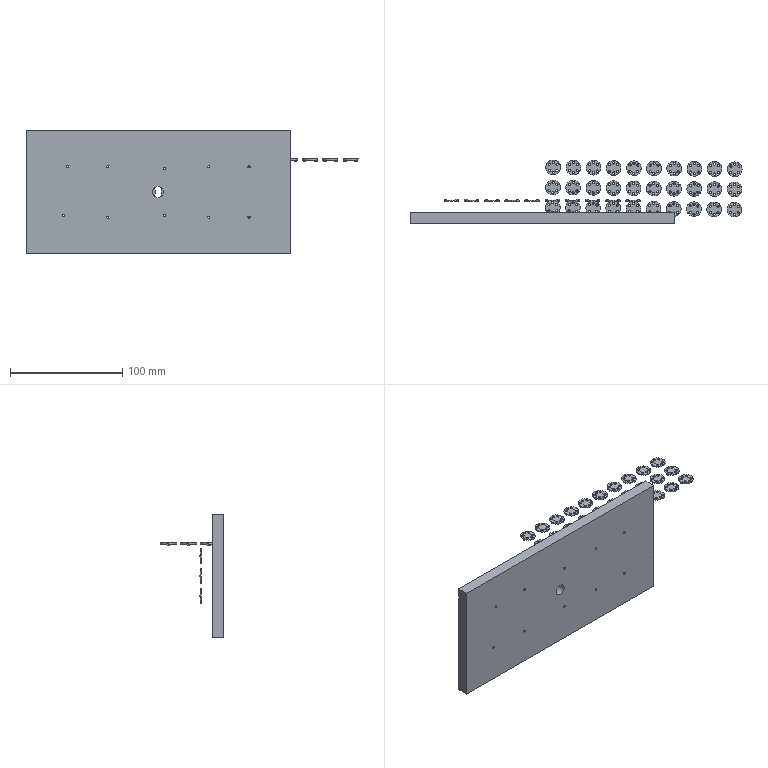CAM job | NX | 3+2 milling, drilling | part box 296.27 x 56.878 x 110 mm
Tools:
number,name,description,diameter,corner_radius,flute_length,length,flutes
0,D10R0,Milling Tool-5 Parameters,10.0,0.0,50.0,75.0,2
0,D3.R0,Milling Tool-5 Parameters,3.0,0.0,50.0,75.0,2
0,DK-Ø3,Countersink,3.0,0.0,0.0,60.0,2
0,D02钻头,Drilling Tool,2.0,0.0,35.0,50.0,2
0,D5R0,Milling Tool-5 Parameters,5.0,0.0,50.0,75.0,2
0,DJ-Ø3,Countersink,3.0,0.0,0.0,60.0,2
0,D2R0,Milling Tool-5 Parameters,2.0,0.0,50.0,75.0,2
0,DK-Ø6,Countersink,6.0,0.0,0.0,60.0,2
15,D16,Milling Tool-5 Parameters,16.0,0.0,50.0,75.0,2
9,D1,Milling Tool-5 Parameters,1.0,0.0,50.0,75.0,2
10,Z2.,Drilling Tool,2.0,0.0,35.0,50.0,2
Operations:
program,operation,operation_type,tool,method,geometry_group,spindle_rpm,surface_speed,feed_per_tooth,feed_cut,feed_plunge,cut_length_mm,path_length_mm,cut_time_min,machine_time_min
B01,FACE_MILLING_1,FaceMilling,D10R0,METHOD,WORKPIECE,2200.0,69.0,0.2727,1200.0,100.0,4849.667,5012.378,4.041,4.061
B02,FACE_MILLING_1_COPY,FaceMilling,D10R0,METHOD,WORKPIECE,2200.0,69.0,0.1818,800.0,100.0,1616.556,1637.456,2.021,2.024
B03,CAVITY_MILL_2,CavityMilling,D3.R0,METHOD,WORKPIECE,4000.0,50.0,0.25,2000.0,100.0,20644.369,20676.269,10.322,10.326
B04,DRILLING,Operation,DK-Ø3,METHOD,WORKPIECE,1500.0,14.0,0.0333,100.0,0.0,360.0,3355.57,3.6,3.9
B04,PLANAR_MILL_COPY_1_COPY_10,PlanarMilling,DK-Ø3,METHOD,WORKPIECE,5000.0,47.0,0.08,800.0,100.0,1403.867,2145.008,1.755,1.84
B05,DRILLING_COPY,Operation,D02钻头,METHOD,WORKPIECE,1500.0,14.0,0.0333,100.0,0.0,900.0,4435.57,9.0,9.354
B06,PLANAR_MILL_3,PlanarMilling,D16,METHOD,WORKPIECE,3500.0,175.0,0.0571,400.0,100.0,639.0,1096.562,1.597,1.643
A01,FACE_MILLING_1_COPY_1,FaceMilling,D10R0,METHOD,WORKPIECE_1,2200.0,69.0,0.2727,1200.0,100.0,4077.75,4637.993,3.398,3.461
A01,FACE_MILLING_1_COPY_1_COPY,FaceMilling,D10R0,METHOD,WORKPIECE_1,2500.0,78.0,0.14,700.0,100.0,1359.25,1459.25,1.942,1.957
A01,PLANAR_MILL_1,PlanarMilling,D10R0,METHOD,WORKPIECE_1,2500.0,78.0,0.14,700.0,100.0,2997.729,3611.928,4.282,4.344
A02,CAVITY_MILL_1_1,CavityMilling,D5R0,METHOD,WORKPIECE_1,4000.0,62.0,0.125,1000.0,100.0,21064.46,21624.203,21.064,21.123
A03,PLANAR_MILL_1_COPY_31,PlanarMilling,D1,METHOD,WORKPIECE_1,4500.0,14.0,0.0667,600.0,100.0,240.132,248.632,0.4002,0.4011
A03,PLANAR_MILL_1_COPY_COPY_30,PlanarMilling,D1,METHOD,WORKPIECE_1,4500.0,14.0,0.0667,600.0,100.0,240.132,248.632,0.4002,0.4011
A03,PLANAR_MILL_1_COPY_31_COPY_1,PlanarMilling,D1,METHOD,WORKPIECE_1,4500.0,14.0,0.0667,600.0,100.0,240.132,248.632,0.4002,0.4011
A03,PLANAR_MILL_1_COPY_COPY_30_COPY_1,PlanarMilling,D1,METHOD,WORKPIECE_1,4500.0,14.0,0.0667,600.0,100.0,240.132,248.632,0.4002,0.4011
A03,PLANAR_MILL_1_COPY_31_COPY_2,PlanarMilling,D1,METHOD,WORKPIECE_1,4500.0,14.0,0.0667,600.0,100.0,240.132,248.632,0.4002,0.4011
A03,PLANAR_MILL_1_COPY_COPY_30_COPY_2,PlanarMilling,D1,METHOD,WORKPIECE_1,4500.0,14.0,0.0667,600.0,100.0,240.132,248.632,0.4002,0.4011
A03,PLANAR_MILL_1_COPY_31_COPY_3,PlanarMilling,D1,METHOD,WORKPIECE_1,4500.0,14.0,0.0667,600.0,100.0,240.132,248.632,0.4002,0.4011
A03,PLANAR_MILL_1_COPY_COPY_30_COPY_3,PlanarMilling,D1,METHOD,WORKPIECE_1,4500.0,14.0,0.0667,600.0,100.0,240.132,248.632,0.4002,0.4011
A03,PLANAR_MILL_1_COPY_31_COPY_4,PlanarMilling,D1,METHOD,WORKPIECE_1,4500.0,14.0,0.0667,600.0,100.0,240.132,248.632,0.4002,0.4011
A03,PLANAR_MILL_1_COPY_COPY_30_COPY_4,PlanarMilling,D1,METHOD,WORKPIECE_1,4500.0,14.0,0.0667,600.0,100.0,240.132,248.632,0.4002,0.4011
A03,PLANAR_MILL_1_COPY_31_COPY_5,PlanarMilling,D1,METHOD,WORKPIECE_1,4500.0,14.0,0.0667,600.0,100.0,240.132,248.632,0.4002,0.4011
A03,PLANAR_MILL_1_COPY_COPY_30_COPY_5,PlanarMilling,D1,METHOD,WORKPIECE_1,4500.0,14.0,0.0667,600.0,100.0,240.132,248.632,0.4002,0.4011
A03,PLANAR_MILL_1_COPY_31_COPY_6,PlanarMilling,D1,METHOD,WORKPIECE_1,4500.0,14.0,0.0667,600.0,100.0,240.132,248.632,0.4002,0.4011
A03,PLANAR_MILL_1_COPY_COPY_30_COPY_6,PlanarMilling,D1,METHOD,WORKPIECE_1,4500.0,14.0,0.0667,600.0,100.0,240.132,248.632,0.4002,0.4011
A03,PLANAR_MILL_1_COPY_31_COPY_7,PlanarMilling,D1,METHOD,WORKPIECE_1,4500.0,14.0,0.0667,600.0,100.0,240.132,248.632,0.4002,0.4011
A03,PLANAR_MILL_1_COPY_COPY_30_COPY_7,PlanarMilling,D1,METHOD,WORKPIECE_1,4500.0,14.0,0.0667,600.0,100.0,240.132,248.632,0.4002,0.4011
A03,PLANAR_MILL_1_COPY_31_COPY_8,PlanarMilling,D1,METHOD,WORKPIECE_1,4500.0,14.0,0.0667,600.0,100.0,240.132,248.632,0.4002,0.4011
A03,PLANAR_MILL_1_COPY_COPY_30_COPY_8,PlanarMilling,D1,METHOD,WORKPIECE_1,4500.0,14.0,0.0667,600.0,100.0,240.132,248.632,0.4002,0.4011
A03,PLANAR_MILL_1_COPY_31_COPY_9,PlanarMilling,D1,METHOD,WORKPIECE_1,4500.0,14.0,0.0667,600.0,100.0,240.132,248.632,0.4002,0.4011
A03,PLANAR_MILL_1_COPY_COPY_30_COPY_9,PlanarMilling,D1,METHOD,WORKPIECE_1,4500.0,14.0,0.0667,600.0,100.0,240.132,248.632,0.4002,0.4011
A03,PLANAR_MILL_1_COPY_31_COPY_10,PlanarMilling,D1,METHOD,WORKPIECE_1,4500.0,14.0,0.0667,600.0,100.0,240.132,248.632,0.4002,0.4011
A03,PLANAR_MILL_1_COPY_COPY_30_COPY_10,PlanarMilling,D1,METHOD,WORKPIECE_1,4500.0,14.0,0.0667,600.0,100.0,240.132,248.632,0.4002,0.4011
A03,PLANAR_MILL_1_COPY_31_COPY_11,PlanarMilling,D1,METHOD,WORKPIECE_1,4500.0,14.0,0.0667,600.0,100.0,240.132,248.632,0.4002,0.4011
A03,PLANAR_MILL_1_COPY_COPY_30_COPY_11,PlanarMilling,D1,METHOD,WORKPIECE_1,4500.0,14.0,0.0667,600.0,100.0,240.132,248.632,0.4002,0.4011
A03,PLANAR_MILL_1_COPY_31_COPY_12,PlanarMilling,D1,METHOD,WORKPIECE_1,4500.0,14.0,0.0667,600.0,100.0,240.132,248.632,0.4002,0.4011
A03,PLANAR_MILL_1_COPY_COPY_30_COPY_12,PlanarMilling,D1,METHOD,WORKPIECE_1,4500.0,14.0,0.0667,600.0,100.0,240.132,248.632,0.4002,0.4011
A03,PLANAR_MILL_1_COPY_31_COPY_13,PlanarMilling,D1,METHOD,WORKPIECE_1,4500.0,14.0,0.0667,600.0,100.0,240.132,248.632,0.4002,0.4011
A03,PLANAR_MILL_1_COPY_COPY_30_COPY_13,PlanarMilling,D1,METHOD,WORKPIECE_1,4500.0,14.0,0.0667,600.0,100.0,240.132,248.632,0.4002,0.4011
A03,PLANAR_MILL_1_COPY_31_COPY_14,PlanarMilling,D1,METHOD,WORKPIECE_1,4500.0,14.0,0.0667,600.0,100.0,240.132,248.632,0.4002,0.4011
A03,PLANAR_MILL_1_COPY_COPY_30_COPY_14,PlanarMilling,D1,METHOD,WORKPIECE_1,4500.0,14.0,0.0667,600.0,100.0,240.132,248.632,0.4002,0.4011
A03,PLANAR_MILL_1_COPY_31_COPY_15,PlanarMilling,D1,METHOD,WORKPIECE_1,4500.0,14.0,0.0667,600.0,100.0,240.132,248.632,0.4002,0.4011
A03,PLANAR_MILL_1_COPY_COPY_30_COPY_15,PlanarMilling,D1,METHOD,WORKPIECE_1,4500.0,14.0,0.0667,600.0,100.0,240.132,248.632,0.4002,0.4011
A03,PLANAR_MILL_1_COPY_31_COPY_16,PlanarMilling,D1,METHOD,WORKPIECE_1,4500.0,14.0,0.0667,600.0,100.0,240.132,248.632,0.4002,0.4011
A03,PLANAR_MILL_1_COPY_COPY_30_COPY_16,PlanarMilling,D1,METHOD,WORKPIECE_1,4500.0,14.0,0.0667,600.0,100.0,240.132,248.632,0.4002,0.4011
A03,PLANAR_MILL_1_COPY_31_COPY_17,PlanarMilling,D1,METHOD,WORKPIECE_1,4500.0,14.0,0.0667,600.0,100.0,240.132,248.632,0.4002,0.4011
A03,PLANAR_MILL_1_COPY_COPY_30_COPY_17,PlanarMilling,D1,METHOD,WORKPIECE_1,4500.0,14.0,0.0667,600.0,100.0,240.132,248.632,0.4002,0.4011
A03,PLANAR_MILL_1_COPY_31_COPY_18,PlanarMilling,D1,METHOD,WORKPIECE_1,4500.0,14.0,0.0667,600.0,100.0,240.132,248.632,0.4002,0.4011
A03,PLANAR_MILL_1_COPY_COPY_30_COPY_18,PlanarMilling,D1,METHOD,WORKPIECE_1,4500.0,14.0,0.0667,600.0,100.0,240.132,248.632,0.4002,0.4011
A03,PLANAR_MILL_1_COPY_31_COPY_19,PlanarMilling,D1,METHOD,WORKPIECE_1,4500.0,14.0,0.0667,600.0,100.0,240.132,248.632,0.4002,0.4011
A03,PLANAR_MILL_1_COPY_COPY_30_COPY_19,PlanarMilling,D1,METHOD,WORKPIECE_1,4500.0,14.0,0.0667,600.0,100.0,240.132,248.632,0.4002,0.4011
A03,PLANAR_MILL_1_COPY_31_COPY_20,PlanarMilling,D1,METHOD,WORKPIECE_1,4500.0,14.0,0.0667,600.0,100.0,240.132,248.632,0.4002,0.4011
A03,PLANAR_MILL_1_COPY_COPY_30_COPY_20,PlanarMilling,D1,METHOD,WORKPIECE_1,4500.0,14.0,0.0667,600.0,100.0,240.132,248.632,0.4002,0.4011
A03,PLANAR_MILL_1_COPY_31_COPY_21,PlanarMilling,D1,METHOD,WORKPIECE_1,4500.0,14.0,0.0667,600.0,100.0,240.132,248.632,0.4002,0.4011
A03,PLANAR_MILL_1_COPY_COPY_30_COPY_21,PlanarMilling,D1,METHOD,WORKPIECE_1,4500.0,14.0,0.0667,600.0,100.0,240.132,248.632,0.4002,0.4011
A03,PLANAR_MILL_1_COPY_31_COPY_22,PlanarMilling,D1,METHOD,WORKPIECE_1,4500.0,14.0,0.0667,600.0,100.0,240.132,248.632,0.4002,0.4011
A03,PLANAR_MILL_1_COPY_COPY_30_COPY_22,PlanarMilling,D1,METHOD,WORKPIECE_1,4500.0,14.0,0.0667,600.0,100.0,240.132,248.632,0.4002,0.4011
A03,PLANAR_MILL_1_COPY_31_COPY_23,PlanarMilling,D1,METHOD,WORKPIECE_1,4500.0,14.0,0.0667,600.0,100.0,240.132,248.632,0.4002,0.4011
A03,PLANAR_MILL_1_COPY_COPY_30_COPY_23,PlanarMilling,D1,METHOD,WORKPIECE_1,4500.0,14.0,0.0667,600.0,100.0,240.132,248.632,0.4002,0.4011
A03,PLANAR_MILL_1_COPY_31_COPY_24,PlanarMilling,D1,METHOD,WORKPIECE_1,4500.0,14.0,0.0667,600.0,100.0,240.132,248.632,0.4002,0.4011
A03,PLANAR_MILL_1_COPY_COPY_30_COPY_24,PlanarMilling,D1,METHOD,WORKPIECE_1,4500.0,14.0,0.0667,600.0,100.0,240.132,248.632,0.4002,0.4011
A03,PLANAR_MILL_1_COPY_31_COPY_25,PlanarMilling,D1,METHOD,WORKPIECE_1,4500.0,14.0,0.0667,600.0,100.0,240.132,248.632,0.4002,0.4011
A03,PLANAR_MILL_1_COPY_COPY_30_COPY_25,PlanarMilling,D1,METHOD,WORKPIECE_1,4500.0,14.0,0.0667,600.0,100.0,240.132,248.632,0.4002,0.4011
A03,PLANAR_MILL_1_COPY_31_COPY_26,PlanarMilling,D1,METHOD,WORKPIECE_1,4500.0,14.0,0.0667,600.0,100.0,240.132,248.632,0.4002,0.4011
A03,PLANAR_MILL_1_COPY_COPY_30_COPY_26,PlanarMilling,D1,METHOD,WORKPIECE_1,4500.0,14.0,0.0667,600.0,100.0,240.132,248.632,0.4002,0.4011
A03,PLANAR_MILL_1_COPY_31_COPY_27,PlanarMilling,D1,METHOD,WORKPIECE_1,4500.0,14.0,0.0667,600.0,100.0,240.132,248.632,0.4002,0.4011
A03,PLANAR_MILL_1_COPY_COPY_30_COPY_27,PlanarMilling,D1,METHOD,WORKPIECE_1,4500.0,14.0,0.0667,600.0,100.0,240.132,248.632,0.4002,0.4011
A03,PLANAR_MILL_1_COPY_31_COPY_28,PlanarMilling,D1,METHOD,WORKPIECE_1,4500.0,14.0,0.0667,600.0,100.0,240.132,248.632,0.4002,0.4011
A03,PLANAR_MILL_1_COPY_COPY_30_COPY_28,PlanarMilling,D1,METHOD,WORKPIECE_1,4500.0,14.0,0.0667,600.0,100.0,240.132,248.632,0.4002,0.4011
A03,PLANAR_MILL_1_COPY_31_COPY_29,PlanarMilling,D1,METHOD,WORKPIECE_1,4500.0,14.0,0.0667,600.0,100.0,240.132,248.632,0.4002,0.4011
A03,PLANAR_MILL_1_COPY_COPY_30_COPY_29,PlanarMilling,D1,METHOD,WORKPIECE_1,4500.0,14.0,0.0667,600.0,100.0,240.132,248.632,0.4002,0.4011
A04,PLANAR_MILL,PlanarMilling,D5R0,METHOD,WORKPIECE_1,3500.0,54.0,0.0286,200.0,100.0,63.307,66.307,0.3165,0.317
A04,PLANAR_MILL_COPY,PlanarMilling,D5R0,METHOD,WORKPIECE_1,3500.0,54.0,0.0286,200.0,100.0,55.6,68.112,0.278,0.2794
A04,PLANAR_MILL_COPY_1,PlanarMilling,D5R0,METHOD,WORKPIECE_1,3500.0,54.0,0.0286,200.0,100.0,63.307,66.307,0.3165,0.317
A04,PLANAR_MILL_COPY_COPY,PlanarMilling,D5R0,METHOD,WORKPIECE_1,3500.0,54.0,0.0286,200.0,100.0,55.6,68.112,0.278,0.2794
A04,PLANAR_MILL_COPY_2,PlanarMilling,D5R0,METHOD,WORKPIECE_1,3500.0,54.0,0.0286,200.0,100.0,63.307,66.307,0.3165,0.317
A04,PLANAR_MILL_COPY_COPY_1,PlanarMilling,D5R0,METHOD,WORKPIECE_1,3500.0,54.0,0.0286,200.0,100.0,55.6,68.112,0.278,0.2794
A04,PLANAR_MILL_COPY_3,PlanarMilling,D5R0,METHOD,WORKPIECE_1,3500.0,54.0,0.0286,200.0,100.0,63.307,66.307,0.3165,0.317
A04,PLANAR_MILL_COPY_COPY_2,PlanarMilling,D5R0,METHOD,WORKPIECE_1,3500.0,54.0,0.0286,200.0,100.0,55.6,68.112,0.278,0.2794
A04,PLANAR_MILL_COPY_4,PlanarMilling,D5R0,METHOD,WORKPIECE_1,3500.0,54.0,0.0286,200.0,100.0,63.307,66.307,0.3165,0.317
A04,PLANAR_MILL_COPY_COPY_3,PlanarMilling,D5R0,METHOD,WORKPIECE_1,3500.0,54.0,0.0286,200.0,100.0,55.6,68.112,0.278,0.2794
A04,PLANAR_MILL_COPY_5,PlanarMilling,D5R0,METHOD,WORKPIECE_1,3500.0,54.0,0.0286,200.0,100.0,63.307,66.307,0.3165,0.317
A04,PLANAR_MILL_COPY_COPY_4,PlanarMilling,D5R0,METHOD,WORKPIECE_1,3500.0,54.0,0.0286,200.0,100.0,55.6,68.112,0.278,0.2794
A04,PLANAR_MILL_COPY_6,PlanarMilling,D5R0,METHOD,WORKPIECE_1,3500.0,54.0,0.0286,200.0,100.0,63.307,66.307,0.3165,0.317
A04,PLANAR_MILL_COPY_COPY_5,PlanarMilling,D5R0,METHOD,WORKPIECE_1,3500.0,54.0,0.0286,200.0,100.0,55.6,68.112,0.278,0.2794
A04,PLANAR_MILL_COPY_7,PlanarMilling,D5R0,METHOD,WORKPIECE_1,3500.0,54.0,0.0286,200.0,100.0,63.307,66.307,0.3165,0.317
A04,PLANAR_MILL_COPY_COPY_6,PlanarMilling,D5R0,METHOD,WORKPIECE_1,3500.0,54.0,0.0286,200.0,100.0,55.6,68.112,0.278,0.2794
A04,PLANAR_MILL_COPY_8,PlanarMilling,D5R0,METHOD,WORKPIECE_1,3500.0,54.0,0.0286,200.0,100.0,63.307,66.307,0.3165,0.317
A04,PLANAR_MILL_COPY_COPY_7,PlanarMilling,D5R0,METHOD,WORKPIECE_1,3500.0,54.0,0.0286,200.0,100.0,55.6,68.112,0.278,0.2794
A04,PLANAR_MILL_COPY_9,PlanarMilling,D5R0,METHOD,WORKPIECE_1,3500.0,54.0,0.0286,200.0,100.0,63.307,66.307,0.3165,0.317
A04,PLANAR_MILL_COPY_COPY_8,PlanarMilling,D5R0,METHOD,WORKPIECE_1,3500.0,54.0,0.0286,200.0,100.0,55.6,68.112,0.278,0.2794
A04,PLANAR_MILL_COPY_10,PlanarMilling,D5R0,METHOD,WORKPIECE_1,3500.0,54.0,0.0286,200.0,100.0,63.307,66.307,0.3165,0.317
A04,PLANAR_MILL_COPY_COPY_9,PlanarMilling,D5R0,METHOD,WORKPIECE_1,3500.0,54.0,0.0286,200.0,100.0,55.6,68.112,0.278,0.2794
A04,PLANAR_MILL_COPY_1_COPY_1,PlanarMilling,D5R0,METHOD,WORKPIECE_1,3500.0,54.0,0.0286,200.0,100.0,63.307,66.307,0.3165,0.317
A04,PLANAR_MILL_COPY_COPY_COPY,PlanarMilling,D5R0,METHOD,WORKPIECE_1,3500.0,54.0,0.0286,200.0,100.0,55.6,68.112,0.278,0.2794
A04,PLANAR_MILL_COPY_2_COPY,PlanarMilling,D5R0,METHOD,WORKPIECE_1,3500.0,54.0,0.0286,200.0,100.0,63.307,66.307,0.3165,0.317
A04,PLANAR_MILL_COPY_COPY_1_COPY,PlanarMilling,D5R0,METHOD,WORKPIECE_1,3500.0,54.0,0.0286,200.0,100.0,55.6,68.112,0.278,0.2794
A04,PLANAR_MILL_COPY_3_COPY,PlanarMilling,D5R0,METHOD,WORKPIECE_1,3500.0,54.0,0.0286,200.0,100.0,63.307,66.307,0.3165,0.317
A04,PLANAR_MILL_COPY_COPY_2_COPY,PlanarMilling,D5R0,METHOD,WORKPIECE_1,3500.0,54.0,0.0286,200.0,100.0,55.6,68.112,0.278,0.2794
A04,PLANAR_MILL_COPY_4_COPY,PlanarMilling,D5R0,METHOD,WORKPIECE_1,3500.0,54.0,0.0286,200.0,100.0,63.307,66.307,0.3165,0.317
A04,PLANAR_MILL_COPY_COPY_3_COPY,PlanarMilling,D5R0,METHOD,WORKPIECE_1,3500.0,54.0,0.0286,200.0,100.0,55.6,68.112,0.278,0.2794
A04,PLANAR_MILL_COPY_5_COPY,PlanarMilling,D5R0,METHOD,WORKPIECE_1,3500.0,54.0,0.0286,200.0,100.0,63.307,66.307,0.3165,0.317
A04,PLANAR_MILL_COPY_COPY_4_COPY,PlanarMilling,D5R0,METHOD,WORKPIECE_1,3500.0,54.0,0.0286,200.0,100.0,55.6,68.112,0.278,0.2794
A04,PLANAR_MILL_COPY_6_COPY,PlanarMilling,D5R0,METHOD,WORKPIECE_1,3500.0,54.0,0.0286,200.0,100.0,63.307,66.307,0.3165,0.317
A04,PLANAR_MILL_COPY_COPY_5_COPY,PlanarMilling,D5R0,METHOD,WORKPIECE_1,3500.0,54.0,0.0286,200.0,100.0,55.6,68.112,0.278,0.2794
A04,PLANAR_MILL_COPY_7_COPY,PlanarMilling,D5R0,METHOD,WORKPIECE_1,3500.0,54.0,0.0286,200.0,100.0,63.307,66.307,0.3165,0.317
A04,PLANAR_MILL_COPY_COPY_6_COPY,PlanarMilling,D5R0,METHOD,WORKPIECE_1,3500.0,54.0,0.0286,200.0,100.0,55.6,68.112,0.278,0.2794
A04,PLANAR_MILL_COPY_8_COPY,PlanarMilling,D5R0,METHOD,WORKPIECE_1,3500.0,54.0,0.0286,200.0,100.0,63.307,66.307,0.3165,0.317
A04,PLANAR_MILL_COPY_COPY_7_COPY,PlanarMilling,D5R0,METHOD,WORKPIECE_1,3500.0,54.0,0.0286,200.0,100.0,55.6,68.112,0.278,0.2794
A04,PLANAR_MILL_COPY_9_COPY,PlanarMilling,D5R0,METHOD,WORKPIECE_1,3500.0,54.0,0.0286,200.0,100.0,63.307,66.307,0.3165,0.317
A04,PLANAR_MILL_COPY_COPY_8_COPY,PlanarMilling,D5R0,METHOD,WORKPIECE_1,3500.0,54.0,0.0286,200.0,100.0,55.6,68.112,0.278,0.2794
A04,PLANAR_MILL_COPY_11,PlanarMilling,D5R0,METHOD,WORKPIECE_1,3500.0,54.0,0.0286,200.0,100.0,63.307,66.307,0.3165,0.317
A04,PLANAR_MILL_COPY_COPY_10,PlanarMilling,D5R0,METHOD,WORKPIECE_1,3500.0,54.0,0.0286,200.0,100.0,55.6,68.112,0.278,0.2794
A04,PLANAR_MILL_COPY_1_COPY_2,PlanarMilling,D5R0,METHOD,WORKPIECE_1,3500.0,54.0,0.0286,200.0,100.0,63.307,66.307,0.3165,0.317
A04,PLANAR_MILL_COPY_COPY_COPY_1,PlanarMilling,D5R0,METHOD,WORKPIECE_1,3500.0,54.0,0.0286,200.0,100.0,55.6,68.112,0.278,0.2794
A04,PLANAR_MILL_COPY_2_COPY_1,PlanarMilling,D5R0,METHOD,WORKPIECE_1,3500.0,54.0,0.0286,200.0,100.0,63.307,66.307,0.3165,0.317
A04,PLANAR_MILL_COPY_COPY_1_COPY_1,PlanarMilling,D5R0,METHOD,WORKPIECE_1,3500.0,54.0,0.0286,200.0,100.0,55.6,68.112,0.278,0.2794
A04,PLANAR_MILL_COPY_3_COPY_1,PlanarMilling,D5R0,METHOD,WORKPIECE_1,3500.0,54.0,0.0286,200.0,100.0,63.307,66.307,0.3165,0.317
A04,PLANAR_MILL_COPY_COPY_2_COPY_1,PlanarMilling,D5R0,METHOD,WORKPIECE_1,3500.0,54.0,0.0286,200.0,100.0,55.6,68.112,0.278,0.2794
A04,PLANAR_MILL_COPY_4_COPY_1,PlanarMilling,D5R0,METHOD,WORKPIECE_1,3500.0,54.0,0.0286,200.0,100.0,63.307,66.307,0.3165,0.317
A04,PLANAR_MILL_COPY_COPY_3_COPY_1,PlanarMilling,D5R0,METHOD,WORKPIECE_1,3500.0,54.0,0.0286,200.0,100.0,55.6,68.112,0.278,0.2794
A04,PLANAR_MILL_COPY_5_COPY_1,PlanarMilling,D5R0,METHOD,WORKPIECE_1,3500.0,54.0,0.0286,200.0,100.0,63.307,66.307,0.3165,0.317
A04,PLANAR_MILL_COPY_COPY_4_COPY_1,PlanarMilling,D5R0,METHOD,WORKPIECE_1,3500.0,54.0,0.0286,200.0,100.0,55.6,68.112,0.278,0.2794
A04,PLANAR_MILL_COPY_6_COPY_1,PlanarMilling,D5R0,METHOD,WORKPIECE_1,3500.0,54.0,0.0286,200.0,100.0,63.307,66.307,0.3165,0.317
A04,PLANAR_MILL_COPY_COPY_5_COPY_1,PlanarMilling,D5R0,METHOD,WORKPIECE_1,3500.0,54.0,0.0286,200.0,100.0,55.6,68.112,0.278,0.2794
A04,PLANAR_MILL_COPY_7_COPY_1,PlanarMilling,D5R0,METHOD,WORKPIECE_1,3500.0,54.0,0.0286,200.0,100.0,63.307,66.307,0.3165,0.317
A04,PLANAR_MILL_COPY_COPY_6_COPY_1,PlanarMilling,D5R0,METHOD,WORKPIECE_1,3500.0,54.0,0.0286,200.0,100.0,55.6,68.112,0.278,0.2794
A04,PLANAR_MILL_COPY_8_COPY_1,PlanarMilling,D5R0,METHOD,WORKPIECE_1,3500.0,54.0,0.0286,200.0,100.0,63.307,66.307,0.3165,0.317
A04,PLANAR_MILL_COPY_COPY_7_COPY_1,PlanarMilling,D5R0,METHOD,WORKPIECE_1,3500.0,54.0,0.0286,200.0,100.0,55.6,68.112,0.278,0.2794
A04,PLANAR_MILL_COPY_9_COPY_1,PlanarMilling,D5R0,METHOD,WORKPIECE_1,3500.0,54.0,0.0286,200.0,100.0,63.307,66.307,0.3165,0.317
A04,PLANAR_MILL_COPY_COPY_8_COPY_1,PlanarMilling,D5R0,METHOD,WORKPIECE_1,3500.0,54.0,0.0286,200.0,100.0,55.6,68.112,0.278,0.2794
A06,CAVITY_MILL_1,CavityMilling,D3.R0,METHOD,WORKPIECE_2,4000.0,50.0,0.25,2000.0,100.0,21910.472,21937.592,10.955,10.96
A06,PLANAR_MILL_2,PlanarMilling,D3.R0,METHOD,WORKPIECE_1,4000.0,50.0,0.075,600.0,100.0,56.236,156.336,0.0937,0.1037
A06,PLANAR_MILL_2_COPY_1,PlanarMilling,D3.R0,METHOD,WORKPIECE_1,4000.0,50.0,0.075,600.0,100.0,56.236,156.336,0.0937,0.1037
A06,PLANAR_MILL_2_COPY_2,PlanarMilling,D3.R0,METHOD,WORKPIECE_1,4000.0,50.0,0.075,600.0,100.0,56.236,156.336,0.0937,0.1037
A06,PLANAR_MILL_2_COPY_3,PlanarMilling,D3.R0,METHOD,WORKPIECE_1,4000.0,50.0,0.075,600.0,100.0,56.236,156.336,0.0937,0.1037
A06,PLANAR_MILL_2_COPY_4,PlanarMilling,D3.R0,METHOD,WORKPIECE_1,4000.0,50.0,0.075,600.0,100.0,56.236,156.336,0.0937,0.1037
A06,PLANAR_MILL_2_COPY_5,PlanarMilling,D3.R0,METHOD,WORKPIECE_1,4000.0,50.0,0.075,600.0,100.0,56.236,156.336,0.0937,0.1037
A06,PLANAR_MILL_2_COPY_6,PlanarMilling,D3.R0,METHOD,WORKPIECE_1,4000.0,50.0,0.075,600.0,100.0,56.236,156.336,0.0937,0.1037
A06,PLANAR_MILL_2_COPY_7,PlanarMilling,D3.R0,METHOD,WORKPIECE_1,4000.0,50.0,0.075,600.0,100.0,56.236,156.336,0.0937,0.1037
A06,PLANAR_MILL_2_COPY_8,PlanarMilling,D3.R0,METHOD,WORKPIECE_1,4000.0,50.0,0.075,600.0,100.0,56.236,156.336,0.0937,0.1037
A06,PLANAR_MILL_2_COPY_9,PlanarMilling,D3.R0,METHOD,WORKPIECE_1,4000.0,50.0,0.075,600.0,100.0,56.236,156.336,0.0937,0.1037
A06,PLANAR_MILL_2_COPY_10,PlanarMilling,D3.R0,METHOD,WORKPIECE_1,4000.0,50.0,0.075,600.0,100.0,56.236,156.336,0.0937,0.1037
A06,PLANAR_MILL_2_COPY_11,PlanarMilling,D3.R0,METHOD,WORKPIECE_1,4000.0,50.0,0.075,600.0,100.0,56.236,156.336,0.0937,0.1037
A06,PLANAR_MILL_2_COPY_12,PlanarMilling,D3.R0,METHOD,WORKPIECE_1,4000.0,50.0,0.075,600.0,100.0,56.236,156.336,0.0937,0.1037
A06,PLANAR_MILL_2_COPY_13,PlanarMilling,D3.R0,METHOD,WORKPIECE_1,4000.0,50.0,0.075,600.0,100.0,56.236,156.336,0.0937,0.1037
A06,PLANAR_MILL_2_COPY_14,PlanarMilling,D3.R0,METHOD,WORKPIECE_1,4000.0,50.0,0.075,600.0,100.0,56.236,156.336,0.0937,0.1037
A06,PLANAR_MILL_2_COPY_15,PlanarMilling,D3.R0,METHOD,WORKPIECE_1,4000.0,50.0,0.075,600.0,100.0,56.236,156.336,0.0937,0.1037
A06,PLANAR_MILL_2_COPY_16,PlanarMilling,D3.R0,METHOD,WORKPIECE_1,4000.0,50.0,0.075,600.0,100.0,56.236,156.336,0.0937,0.1037
A06,PLANAR_MILL_2_COPY_17,PlanarMilling,D3.R0,METHOD,WORKPIECE_1,4000.0,50.0,0.075,600.0,100.0,56.236,156.336,0.0937,0.1037
A06,PLANAR_MILL_2_COPY_18,PlanarMilling,D3.R0,METHOD,WORKPIECE_1,4000.0,50.0,0.075,600.0,100.0,56.236,156.336,0.0937,0.1037
A06,PLANAR_MILL_2_COPY_19,PlanarMilling,D3.R0,METHOD,WORKPIECE_1,4000.0,50.0,0.075,600.0,100.0,56.236,156.336,0.0937,0.1037
A06,PLANAR_MILL_2_COPY_20,PlanarMilling,D3.R0,METHOD,WORKPIECE_1,4000.0,50.0,0.075,600.0,100.0,56.236,156.336,0.0937,0.1037
A06,PLANAR_MILL_2_COPY_21,PlanarMilling,D3.R0,METHOD,WORKPIECE_1,4000.0,50.0,0.075,600.0,100.0,56.236,156.336,0.0937,0.1037
A06,PLANAR_MILL_2_COPY_22,PlanarMilling,D3.R0,METHOD,WORKPIECE_1,4000.0,50.0,0.075,600.0,100.0,56.236,156.336,0.0937,0.1037
A06,PLANAR_MILL_2_COPY_23,PlanarMilling,D3.R0,METHOD,WORKPIECE_1,4000.0,50.0,0.075,600.0,100.0,56.236,156.336,0.0937,0.1037
A06,PLANAR_MILL_2_COPY_24,PlanarMilling,D3.R0,METHOD,WORKPIECE_1,4000.0,50.0,0.075,600.0,100.0,56.236,156.336,0.0937,0.1037
A06,PLANAR_MILL_2_COPY_25,PlanarMilling,D3.R0,METHOD,WORKPIECE_1,4000.0,50.0,0.075,600.0,100.0,56.236,156.336,0.0937,0.1037
A06,PLANAR_MILL_2_COPY_26,PlanarMilling,D3.R0,METHOD,WORKPIECE_1,4000.0,50.0,0.075,600.0,100.0,56.236,156.336,0.0937,0.1037
A06,PLANAR_MILL_2_COPY_27,PlanarMilling,D3.R0,METHOD,WORKPIECE_1,4000.0,50.0,0.075,600.0,100.0,56.236,156.336,0.0937,0.1037
A06,PLANAR_MILL_2_COPY_28,PlanarMilling,D3.R0,METHOD,WORKPIECE_1,4000.0,50.0,0.075,600.0,100.0,56.236,156.336,0.0937,0.1037
A06,PLANAR_MILL_2_COPY_29,PlanarMilling,D3.R0,METHOD,WORKPIECE_1,4000.0,50.0,0.075,600.0,100.0,56.236,156.336,0.0937,0.1037
A07,DRILLING_COPY_1_COPY,Operation,DJ-Ø3,METHOD,WORKPIECE_1,1500.0,14.0,0.0667,200.0,0.0,378.0,3067.179,1.89,2.159
A07,PLANAR_MILL_COPY_1_COPY,PlanarMilling,DJ-Ø3,METHOD,WORKPIECE_1,5000.0,47.0,0.08,800.0,100.0,25.4,43.503,0.0318,0.0339
A07,PLANAR_MILL_COPY_1_COPY_9_COPY,PlanarMilling,DJ-Ø3,METHOD,WORKPIECE_1,5000.0,47.0,0.08,800.0,100.0,40.781,59.278,0.051,0.0535
A07,PLANAR_MILL_COPY_1_COPY_12_COPY,PlanarMilling,DJ-Ø3,METHOD,WORKPIECE_1,5000.0,47.0,0.08,800.0,100.0,25.4,43.503,0.0318,0.0339
A07,PLANAR_MILL_COPY_1_COPY_9_COPY_1_COPY,PlanarMilling,DJ-Ø3,METHOD,WORKPIECE_1,5000.0,47.0,0.08,800.0,100.0,40.781,59.278,0.051,0.0535
A07,PLANAR_MILL_COPY_1_COPY_13_COPY,PlanarMilling,DJ-Ø3,METHOD,WORKPIECE_1,5000.0,47.0,0.08,800.0,100.0,25.4,43.503,0.0318,0.0339
A07,PLANAR_MILL_COPY_1_COPY_9_COPY_2_COPY,PlanarMilling,DJ-Ø3,METHOD,WORKPIECE_1,5000.0,47.0,0.08,800.0,100.0,40.781,59.278,0.051,0.0535
A07,PLANAR_MILL_COPY_1_COPY_14_COPY,PlanarMilling,DJ-Ø3,METHOD,WORKPIECE_1,5000.0,47.0,0.08,800.0,100.0,25.4,43.503,0.0318,0.0339
A07,PLANAR_MILL_COPY_1_COPY_9_COPY_3_COPY,PlanarMilling,DJ-Ø3,METHOD,WORKPIECE_1,5000.0,47.0,0.08,800.0,100.0,40.781,59.278,0.051,0.0535
A07,PLANAR_MILL_COPY_1_COPY_15_COPY,PlanarMilling,DJ-Ø3,METHOD,WORKPIECE_1,5000.0,47.0,0.08,800.0,100.0,25.4,43.503,0.0318,0.0339
A07,PLANAR_MILL_COPY_1_COPY_9_COPY_4_COPY,PlanarMilling,DJ-Ø3,METHOD,WORKPIECE_1,5000.0,47.0,0.08,800.0,100.0,40.781,59.278,0.051,0.0535
A07,PLANAR_MILL_COPY_1_COPY_16_COPY,PlanarMilling,DJ-Ø3,METHOD,WORKPIECE_1,5000.0,47.0,0.08,800.0,100.0,25.4,43.503,0.0318,0.0339
A07,PLANAR_MILL_COPY_1_COPY_9_COPY_5_COPY,PlanarMilling,DJ-Ø3,METHOD,WORKPIECE_1,5000.0,47.0,0.08,800.0,100.0,40.781,59.278,0.051,0.0535
A07,PLANAR_MILL_COPY_1_COPY_17_COPY,PlanarMilling,DJ-Ø3,METHOD,WORKPIECE_1,5000.0,47.0,0.08,800.0,100.0,25.4,43.503,0.0318,0.0339
A07,PLANAR_MILL_COPY_1_COPY_9_COPY_6_COPY,PlanarMilling,DJ-Ø3,METHOD,WORKPIECE_1,5000.0,47.0,0.08,800.0,100.0,40.781,59.278,0.051,0.0535
A07,PLANAR_MILL_COPY_1_COPY_18_COPY,PlanarMilling,DJ-Ø3,METHOD,WORKPIECE_1,5000.0,47.0,0.08,800.0,100.0,25.4,43.503,0.0318,0.0339
A07,PLANAR_MILL_COPY_1_COPY_9_COPY_7_COPY,PlanarMilling,DJ-Ø3,METHOD,WORKPIECE_1,5000.0,47.0,0.08,800.0,100.0,40.781,59.278,0.051,0.0535
A07,PLANAR_MILL_COPY_1_COPY_19_COPY,PlanarMilling,DJ-Ø3,METHOD,WORKPIECE_1,5000.0,47.0,0.08,800.0,100.0,25.4,43.503,0.0318,0.0339
A07,PLANAR_MILL_COPY_1_COPY_9_COPY_8_COPY,PlanarMilling,DJ-Ø3,METHOD,WORKPIECE_1,5000.0,47.0,0.08,800.0,100.0,40.781,59.278,0.051,0.0535
A07,PLANAR_MILL_COPY_1_COPY_20_COPY,PlanarMilling,DJ-Ø3,METHOD,WORKPIECE_1,5000.0,47.0,0.08,800.0,100.0,25.4,43.503,0.0318,0.0339
A07,PLANAR_MILL_COPY_1_COPY_9_COPY_9_COPY,PlanarMilling,DJ-Ø3,METHOD,WORKPIECE_1,5000.0,47.0,0.08,800.0,100.0,40.781,59.278,0.051,0.0535
A07,PLANAR_MILL_COPY_1_COPY_21_COPY,PlanarMilling,DJ-Ø3,METHOD,WORKPIECE_1,5000.0,47.0,0.08,800.0,100.0,25.4,43.503,0.0318,0.0339
A07,PLANAR_MILL_COPY_1_COPY_9_COPY_10_COPY,PlanarMilling,DJ-Ø3,METHOD,WORKPIECE_1,5000.0,47.0,0.08,800.0,100.0,40.781,59.278,0.051,0.0535
A07,PLANAR_MILL_COPY_1_COPY_22_COPY,PlanarMilling,DJ-Ø3,METHOD,WORKPIECE_1,5000.0,47.0,0.08,800.0,100.0,25.4,43.503,0.0318,0.0339
A07,PLANAR_MILL_COPY_1_COPY_9_COPY_11_COPY,PlanarMilling,DJ-Ø3,METHOD,WORKPIECE_1,5000.0,47.0,0.08,800.0,100.0,40.781,59.278,0.051,0.0535
A07,PLANAR_MILL_COPY_1_COPY_23_COPY,PlanarMilling,DJ-Ø3,METHOD,WORKPIECE_1,5000.0,47.0,0.08,800.0,100.0,25.4,43.503,0.0318,0.0339
A07,PLANAR_MILL_COPY_1_COPY_9_COPY_12_COPY,PlanarMilling,DJ-Ø3,METHOD,WORKPIECE_1,5000.0,47.0,0.08,800.0,100.0,40.781,59.278,0.051,0.0535
A07,PLANAR_MILL_COPY_1_COPY_24_COPY,PlanarMilling,DJ-Ø3,METHOD,WORKPIECE_1,5000.0,47.0,0.08,800.0,100.0,25.4,43.503,0.0318,0.0339
A07,PLANAR_MILL_COPY_1_COPY_9_COPY_13_COPY,PlanarMilling,DJ-Ø3,METHOD,WORKPIECE_1,5000.0,47.0,0.08,800.0,100.0,40.781,59.278,0.051,0.0535
A07,PLANAR_MILL_COPY_1_COPY_25_COPY,PlanarMilling,DJ-Ø3,METHOD,WORKPIECE_1,5000.0,47.0,0.08,800.0,100.0,25.4,43.503,0.0318,0.0339
A07,PLANAR_MILL_COPY_1_COPY_9_COPY_14_COPY,PlanarMilling,DJ-Ø3,METHOD,WORKPIECE_1,5000.0,47.0,0.08,800.0,100.0,40.781,59.278,0.051,0.0535
A07,PLANAR_MILL_COPY_1_COPY_26_COPY,PlanarMilling,DJ-Ø3,METHOD,WORKPIECE_1,5000.0,47.0,0.08,800.0,100.0,25.4,43.503,0.0318,0.0339
A07,PLANAR_MILL_COPY_1_COPY_9_COPY_15_COPY,PlanarMilling,DJ-Ø3,METHOD,WORKPIECE_1,5000.0,47.0,0.08,800.0,100.0,40.781,59.278,0.051,0.0535
A07,PLANAR_MILL_COPY_1_COPY_27_COPY,PlanarMilling,DJ-Ø3,METHOD,WORKPIECE_1,5000.0,47.0,0.08,800.0,100.0,25.4,43.503,0.0318,0.0339
A07,PLANAR_MILL_COPY_1_COPY_9_COPY_16_COPY,PlanarMilling,DJ-Ø3,METHOD,WORKPIECE_1,5000.0,47.0,0.08,800.0,100.0,40.781,59.278,0.051,0.0535
A07,PLANAR_MILL_COPY_1_COPY_28_COPY,PlanarMilling,DJ-Ø3,METHOD,WORKPIECE_1,5000.0,47.0,0.08,800.0,100.0,25.4,43.503,0.0318,0.0339
A07,PLANAR_MILL_COPY_1_COPY_9_COPY_17_COPY,PlanarMilling,DJ-Ø3,METHOD,WORKPIECE_1,5000.0,47.0,0.08,800.0,100.0,40.781,59.278,0.051,0.0535
A07,PLANAR_MILL_COPY_1_COPY_29_COPY,PlanarMilling,DJ-Ø3,METHOD,WORKPIECE_1,5000.0,47.0,0.08,800.0,100.0,25.4,43.503,0.0318,0.0339
A07,PLANAR_MILL_COPY_1_COPY_9_COPY_18_COPY,PlanarMilling,DJ-Ø3,METHOD,WORKPIECE_1,5000.0,47.0,0.08,800.0,100.0,40.781,59.278,0.051,0.0535
A07,PLANAR_MILL_COPY_1_COPY_30_COPY,PlanarMilling,DJ-Ø3,METHOD,WORKPIECE_1,5000.0,47.0,0.08,800.0,100.0,25.4,43.503,0.0318,0.0339
A07,PLANAR_MILL_COPY_1_COPY_9_COPY_19_COPY,PlanarMilling,DJ-Ø3,METHOD,WORKPIECE_1,5000.0,47.0,0.08,800.0,100.0,40.781,59.278,0.051,0.0535
A07,PLANAR_MILL_COPY_1_COPY_31_COPY,PlanarMilling,DJ-Ø3,METHOD,WORKPIECE_1,5000.0,47.0,0.08,800.0,100.0,25.4,43.503,0.0318,0.0339
A07,PLANAR_MILL_COPY_1_COPY_9_COPY_20_COPY,PlanarMilling,DJ-Ø3,METHOD,WORKPIECE_1,5000.0,47.0,0.08,800.0,100.0,40.781,59.278,0.051,0.0535
A07,PLANAR_MILL_COPY_1_COPY_32_COPY,PlanarMilling,DJ-Ø3,METHOD,WORKPIECE_1,5000.0,47.0,0.08,800.0,100.0,25.4,43.503,0.0318,0.0339
A07,PLANAR_MILL_COPY_1_COPY_9_COPY_21_COPY,PlanarMilling,DJ-Ø3,METHOD,WORKPIECE_1,5000.0,47.0,0.08,800.0,100.0,40.781,59.278,0.051,0.0535
A07,PLANAR_MILL_COPY_1_COPY_33_COPY,PlanarMilling,DJ-Ø3,METHOD,WORKPIECE_1,5000.0,47.0,0.08,800.0,100.0,25.4,43.503,0.0318,0.0339
A07,PLANAR_MILL_COPY_1_COPY_9_COPY_22_COPY,PlanarMilling,DJ-Ø3,METHOD,WORKPIECE_1,5000.0,47.0,0.08,800.0,100.0,40.781,59.278,0.051,0.0535
A07,PLANAR_MILL_COPY_1_COPY_34_COPY,PlanarMilling,DJ-Ø3,METHOD,WORKPIECE_1,5000.0,47.0,0.08,800.0,100.0,25.4,43.503,0.0318,0.0339
A07,PLANAR_MILL_COPY_1_COPY_9_COPY_23_COPY,PlanarMilling,DJ-Ø3,METHOD,WORKPIECE_1,5000.0,47.0,0.08,800.0,100.0,40.781,59.278,0.051,0.0535
A07,PLANAR_MILL_COPY_1_COPY_35_COPY,PlanarMilling,DJ-Ø3,METHOD,WORKPIECE_1,5000.0,47.0,0.08,800.0,100.0,25.4,43.503,0.0318,0.0339
A07,PLANAR_MILL_COPY_1_COPY_9_COPY_24_COPY,PlanarMilling,DJ-Ø3,METHOD,WORKPIECE_1,5000.0,47.0,0.08,800.0,100.0,40.781,59.278,0.051,0.0535
A07,PLANAR_MILL_COPY_1_COPY_36_COPY,PlanarMilling,DJ-Ø3,METHOD,WORKPIECE_1,5000.0,47.0,0.08,800.0,100.0,25.4,43.503,0.0318,0.0339
A07,PLANAR_MILL_COPY_1_COPY_9_COPY_25_COPY,PlanarMilling,DJ-Ø3,METHOD,WORKPIECE_1,5000.0,47.0,0.08,800.0,100.0,40.781,59.278,0.051,0.0535
A07,PLANAR_MILL_COPY_1_COPY_37_COPY,PlanarMilling,DJ-Ø3,METHOD,WORKPIECE_1,5000.0,47.0,0.08,800.0,100.0,25.4,43.503,0.0318,0.0339
A07,PLANAR_MILL_COPY_1_COPY_9_COPY_26_COPY,PlanarMilling,DJ-Ø3,METHOD,WORKPIECE_1,5000.0,47.0,0.08,800.0,100.0,40.781,59.278,0.051,0.0535
A07,PLANAR_MILL_COPY_1_COPY_38_COPY,PlanarMilling,DJ-Ø3,METHOD,WORKPIECE_1,5000.0,47.0,0.08,800.0,100.0,25.4,43.503,0.0318,0.0339
A07,PLANAR_MILL_COPY_1_COPY_9_COPY_27_COPY,PlanarMilling,DJ-Ø3,METHOD,WORKPIECE_1,5000.0,47.0,0.08,800.0,100.0,40.781,59.278,0.051,0.0535
A07,PLANAR_MILL_COPY_1_COPY_39_COPY,PlanarMilling,DJ-Ø3,METHOD,WORKPIECE_1,5000.0,47.0,0.08,800.0,100.0,25.4,43.503,0.0318,0.0339
A07,PLANAR_MILL_COPY_1_COPY_9_COPY_28_COPY,PlanarMilling,DJ-Ø3,METHOD,WORKPIECE_1,5000.0,47.0,0.08,800.0,100.0,40.781,59.278,0.051,0.0535
A07,PLANAR_MILL_COPY_1_COPY_40_COPY,PlanarMilling,DJ-Ø3,METHOD,WORKPIECE_1,5000.0,47.0,0.08,800.0,100.0,25.4,43.503,0.0318,0.0339
A07,PLANAR_MILL_COPY_1_COPY_9_COPY_29_COPY,PlanarMilling,DJ-Ø3,METHOD,WORKPIECE_1,5000.0,47.0,0.08,800.0,100.0,40.781,59.278,0.051,0.0535
A10,PLANAR_MILL_1_COPY_31_COPY,PlanarMilling,D1,METHOD,WORKPIECE_1,4500.0,14.0,0.0667,600.0,100.0,9.33,17.83,0.0156,0.0164
A10,PLANAR_MILL_1_COPY_COPY_30_COPY,PlanarMilling,D1,METHOD,WORKPIECE_1,4500.0,14.0,0.0667,600.0,100.0,9.33,17.83,0.0156,0.0164
A10,PLANAR_MILL_1_COPY_31_COPY_COPY,PlanarMilling,D1,METHOD,WORKPIECE_1,4500.0,14.0,0.0667,600.0,100.0,9.33,17.83,0.0156,0.0164
A10,PLANAR_MILL_1_COPY_COPY_30_COPY_COPY,PlanarMilling,D1,METHOD,WORKPIECE_1,4500.0,14.0,0.0667,600.0,100.0,9.33,17.83,0.0156,0.0164
A10,PLANAR_MILL_1_COPY_31_COPY_COPY_1,PlanarMilling,D1,METHOD,WORKPIECE_1,4500.0,14.0,0.0667,600.0,100.0,9.33,17.83,0.0156,0.0164
A10,PLANAR_MILL_1_COPY_COPY_30_COPY_COPY_1,PlanarMilling,D1,METHOD,WORKPIECE_1,4500.0,14.0,0.0667,600.0,100.0,9.33,17.83,0.0156,0.0164
A10,PLANAR_MILL_1_COPY_31_COPY_COPY_2,PlanarMilling,D1,METHOD,WORKPIECE_1,4500.0,14.0,0.0667,600.0,100.0,9.33,17.83,0.0156,0.0164
A10,PLANAR_MILL_1_COPY_COPY_30_COPY_COPY_2,PlanarMilling,D1,METHOD,WORKPIECE_1,4500.0,14.0,0.0667,600.0,100.0,9.33,17.83,0.0156,0.0164
A10,PLANAR_MILL_1_COPY_31_COPY_COPY_3,PlanarMilling,D1,METHOD,WORKPIECE_1,4500.0,14.0,0.0667,600.0,100.0,9.33,17.83,0.0156,0.0164
A10,PLANAR_MILL_1_COPY_COPY_30_COPY_COPY_3,PlanarMilling,D1,METHOD,WORKPIECE_1,4500.0,14.0,0.0667,600.0,100.0,9.33,17.83,0.0156,0.0164
A10,PLANAR_MILL_1_COPY_31_COPY_COPY_4,PlanarMilling,D1,METHOD,WORKPIECE_1,4500.0,14.0,0.0667,600.0,100.0,9.33,17.83,0.0156,0.0164
A10,PLANAR_MILL_1_COPY_COPY_30_COPY_COPY_4,PlanarMilling,D1,METHOD,WORKPIECE_1,4500.0,14.0,0.0667,600.0,100.0,9.33,17.83,0.0156,0.0164
A10,PLANAR_MILL_1_COPY_31_COPY_COPY_5,PlanarMilling,D1,METHOD,WORKPIECE_1,4500.0,14.0,0.0667,600.0,100.0,9.33,17.83,0.0156,0.0164
A10,PLANAR_MILL_1_COPY_COPY_30_COPY_COPY_5,PlanarMilling,D1,METHOD,WORKPIECE_1,4500.0,14.0,0.0667,600.0,100.0,9.33,17.83,0.0156,0.0164
A10,PLANAR_MILL_1_COPY_31_COPY_COPY_6,PlanarMilling,D1,METHOD,WORKPIECE_1,4500.0,14.0,0.0667,600.0,100.0,9.33,17.83,0.0156,0.0164
A10,PLANAR_MILL_1_COPY_COPY_30_COPY_COPY_6,PlanarMilling,D1,METHOD,WORKPIECE_1,4500.0,14.0,0.0667,600.0,100.0,9.33,17.83,0.0156,0.0164
A10,PLANAR_MILL_1_COPY_31_COPY_COPY_7,PlanarMilling,D1,METHOD,WORKPIECE_1,4500.0,14.0,0.0667,600.0,100.0,9.33,17.83,0.0156,0.0164
A10,PLANAR_MILL_1_COPY_COPY_30_COPY_COPY_7,PlanarMilling,D1,METHOD,WORKPIECE_1,4500.0,14.0,0.0667,600.0,100.0,9.33,17.83,0.0156,0.0164
A10,PLANAR_MILL_1_COPY_31_COPY_COPY_8,PlanarMilling,D1,METHOD,WORKPIECE_1,4500.0,14.0,0.0667,600.0,100.0,9.33,17.83,0.0156,0.0164
A10,PLANAR_MILL_1_COPY_COPY_30_COPY_COPY_8,PlanarMilling,D1,METHOD,WORKPIECE_1,4500.0,14.0,0.0667,600.0,100.0,9.33,17.83,0.0156,0.0164
A10,PLANAR_MILL_1_COPY_31_COPY_COPY_9,PlanarMilling,D1,METHOD,WORKPIECE_1,4500.0,14.0,0.0667,600.0,100.0,9.33,17.83,0.0156,0.0164
A10,PLANAR_MILL_1_COPY_COPY_30_COPY_COPY_9,PlanarMilling,D1,METHOD,WORKPIECE_1,4500.0,14.0,0.0667,600.0,100.0,9.33,17.83,0.0156,0.0164
A10,PLANAR_MILL_1_COPY_31_COPY_COPY_10,PlanarMilling,D1,METHOD,WORKPIECE_1,4500.0,14.0,0.0667,600.0,100.0,9.33,17.83,0.0156,0.0164
A10,PLANAR_MILL_1_COPY_COPY_30_COPY_COPY_10,PlanarMilling,D1,METHOD,WORKPIECE_1,4500.0,14.0,0.0667,600.0,100.0,9.33,17.83,0.0156,0.0164
A10,PLANAR_MILL_1_COPY_31_COPY_COPY_11,PlanarMilling,D1,METHOD,WORKPIECE_1,4500.0,14.0,0.0667,600.0,100.0,9.33,17.83,0.0156,0.0164
A10,PLANAR_MILL_1_COPY_COPY_30_COPY_COPY_11,PlanarMilling,D1,METHOD,WORKPIECE_1,4500.0,14.0,0.0667,600.0,100.0,9.33,17.83,0.0156,0.0164
A10,PLANAR_MILL_1_COPY_31_COPY_COPY_12,PlanarMilling,D1,METHOD,WORKPIECE_1,4500.0,14.0,0.0667,600.0,100.0,9.33,17.83,0.0156,0.0164
A10,PLANAR_MILL_1_COPY_COPY_30_COPY_COPY_12,PlanarMilling,D1,METHOD,WORKPIECE_1,4500.0,14.0,0.0667,600.0,100.0,9.33,17.83,0.0156,0.0164
A10,PLANAR_MILL_1_COPY_31_COPY_COPY_13,PlanarMilling,D1,METHOD,WORKPIECE_1,4500.0,14.0,0.0667,600.0,100.0,9.33,17.83,0.0156,0.0164
A10,PLANAR_MILL_1_COPY_COPY_30_COPY_COPY_13,PlanarMilling,D1,METHOD,WORKPIECE_1,4500.0,14.0,0.0667,600.0,100.0,9.33,17.83,0.0156,0.0164
A10,PLANAR_MILL_1_COPY_31_COPY_COPY_14,PlanarMilling,D1,METHOD,WORKPIECE_1,4500.0,14.0,0.0667,600.0,100.0,9.33,17.83,0.0156,0.0164
A10,PLANAR_MILL_1_COPY_COPY_30_COPY_COPY_14,PlanarMilling,D1,METHOD,WORKPIECE_1,4500.0,14.0,0.0667,600.0,100.0,9.33,17.83,0.0156,0.0164
A10,PLANAR_MILL_1_COPY_31_COPY_COPY_15,PlanarMilling,D1,METHOD,WORKPIECE_1,4500.0,14.0,0.0667,600.0,100.0,9.33,17.83,0.0156,0.0164
A10,PLANAR_MILL_1_COPY_COPY_30_COPY_COPY_15,PlanarMilling,D1,METHOD,WORKPIECE_1,4500.0,14.0,0.0667,600.0,100.0,9.33,17.83,0.0156,0.0164
A10,PLANAR_MILL_1_COPY_31_COPY_COPY_16,PlanarMilling,D1,METHOD,WORKPIECE_1,4500.0,14.0,0.0667,600.0,100.0,9.33,17.83,0.0156,0.0164
A10,PLANAR_MILL_1_COPY_COPY_30_COPY_COPY_16,PlanarMilling,D1,METHOD,WORKPIECE_1,4500.0,14.0,0.0667,600.0,100.0,9.33,17.83,0.0156,0.0164
A10,PLANAR_MILL_1_COPY_31_COPY_COPY_17,PlanarMilling,D1,METHOD,WORKPIECE_1,4500.0,14.0,0.0667,600.0,100.0,9.33,17.83,0.0156,0.0164
A10,PLANAR_MILL_1_COPY_COPY_30_COPY_COPY_17,PlanarMilling,D1,METHOD,WORKPIECE_1,4500.0,14.0,0.0667,600.0,100.0,9.33,17.83,0.0156,0.0164
A10,PLANAR_MILL_1_COPY_31_COPY_COPY_18,PlanarMilling,D1,METHOD,WORKPIECE_1,4500.0,14.0,0.0667,600.0,100.0,9.33,17.83,0.0156,0.0164
A10,PLANAR_MILL_1_COPY_COPY_30_COPY_COPY_18,PlanarMilling,D1,METHOD,WORKPIECE_1,4500.0,14.0,0.0667,600.0,100.0,9.33,17.83,0.0156,0.0164
A10,PLANAR_MILL_1_COPY_31_COPY_COPY_19,PlanarMilling,D1,METHOD,WORKPIECE_1,4500.0,14.0,0.0667,600.0,100.0,9.33,17.83,0.0156,0.0164
A10,PLANAR_MILL_1_COPY_COPY_30_COPY_COPY_19,PlanarMilling,D1,METHOD,WORKPIECE_1,4500.0,14.0,0.0667,600.0,100.0,9.33,17.83,0.0156,0.0164
A10,PLANAR_MILL_1_COPY_31_COPY_COPY_20,PlanarMilling,D1,METHOD,WORKPIECE_1,4500.0,14.0,0.0667,600.0,100.0,9.33,17.83,0.0156,0.0164
A10,PLANAR_MILL_1_COPY_COPY_30_COPY_COPY_20,PlanarMilling,D1,METHOD,WORKPIECE_1,4500.0,14.0,0.0667,600.0,100.0,9.33,17.83,0.0156,0.0164
A10,PLANAR_MILL_1_COPY_31_COPY_COPY_21,PlanarMilling,D1,METHOD,WORKPIECE_1,4500.0,14.0,0.0667,600.0,100.0,9.33,17.83,0.0156,0.0164
A10,PLANAR_MILL_1_COPY_COPY_30_COPY_COPY_21,PlanarMilling,D1,METHOD,WORKPIECE_1,4500.0,14.0,0.0667,600.0,100.0,9.33,17.83,0.0156,0.0164
A10,PLANAR_MILL_1_COPY_31_COPY_COPY_22,PlanarMilling,D1,METHOD,WORKPIECE_1,4500.0,14.0,0.0667,600.0,100.0,9.33,17.83,0.0156,0.0164
A10,PLANAR_MILL_1_COPY_COPY_30_COPY_COPY_22,PlanarMilling,D1,METHOD,WORKPIECE_1,4500.0,14.0,0.0667,600.0,100.0,9.33,17.83,0.0156,0.0164
A10,PLANAR_MILL_1_COPY_31_COPY_COPY_23,PlanarMilling,D1,METHOD,WORKPIECE_1,4500.0,14.0,0.0667,600.0,100.0,9.33,17.83,0.0156,0.0164
A10,PLANAR_MILL_1_COPY_COPY_30_COPY_COPY_23,PlanarMilling,D1,METHOD,WORKPIECE_1,4500.0,14.0,0.0667,600.0,100.0,9.33,17.83,0.0156,0.0164
A10,PLANAR_MILL_1_COPY_31_COPY_COPY_24,PlanarMilling,D1,METHOD,WORKPIECE_1,4500.0,14.0,0.0667,600.0,100.0,9.33,17.83,0.0156,0.0164
A10,PLANAR_MILL_1_COPY_COPY_30_COPY_COPY_24,PlanarMilling,D1,METHOD,WORKPIECE_1,4500.0,14.0,0.0667,600.0,100.0,9.33,17.83,0.0156,0.0164
A10,PLANAR_MILL_1_COPY_31_COPY_COPY_25,PlanarMilling,D1,METHOD,WORKPIECE_1,4500.0,14.0,0.0667,600.0,100.0,9.33,17.83,0.0156,0.0164
A10,PLANAR_MILL_1_COPY_COPY_30_COPY_COPY_25,PlanarMilling,D1,METHOD,WORKPIECE_1,4500.0,14.0,0.0667,600.0,100.0,9.33,17.83,0.0156,0.0164
A10,PLANAR_MILL_1_COPY_31_COPY_COPY_26,PlanarMilling,D1,METHOD,WORKPIECE_1,4500.0,14.0,0.0667,600.0,100.0,9.33,17.83,0.0156,0.0164
A10,PLANAR_MILL_1_COPY_COPY_30_COPY_COPY_26,PlanarMilling,D1,METHOD,WORKPIECE_1,4500.0,14.0,0.0667,600.0,100.0,9.33,17.83,0.0156,0.0164
A10,PLANAR_MILL_1_COPY_31_COPY_COPY_27,PlanarMilling,D1,METHOD,WORKPIECE_1,4500.0,14.0,0.0667,600.0,100.0,9.33,17.83,0.0156,0.0164
A10,PLANAR_MILL_1_COPY_COPY_30_COPY_COPY_27,PlanarMilling,D1,METHOD,WORKPIECE_1,4500.0,14.0,0.0667,600.0,100.0,9.33,17.83,0.0156,0.0164
A10,PLANAR_MILL_1_COPY_31_COPY_COPY_28,PlanarMilling,D1,METHOD,WORKPIECE_1,4500.0,14.0,0.0667,600.0,100.0,9.33,17.83,0.0156,0.0164
A10,PLANAR_MILL_1_COPY_COPY_30_COPY_COPY_28,PlanarMilling,D1,METHOD,WORKPIECE_1,4500.0,14.0,0.0667,600.0,100.0,9.33,17.83,0.0156,0.0164
A10,PLANAR_MILL_1_COPY_31_COPY_COPY_29,PlanarMilling,D1,METHOD,WORKPIECE_1,4500.0,14.0,0.0667,600.0,100.0,9.33,17.83,0.0156,0.0164
A10,PLANAR_MILL_1_COPY_COPY_30_COPY_COPY_29,PlanarMilling,D1,METHOD,WORKPIECE_1,4500.0,14.0,0.0667,600.0,100.0,9.33,17.83,0.0156,0.0164
C01,FLOOR_WALL,VolumeBased25DMillingOperation,D16,METHOD,WORKPIECE_3,4000.0,201.0,0.125,1000.0,100.0,2631.599,2725.599,2.632,2.641
C01,DRILLING_COPY_2,Operation,DK-Ø6,METHOD,WORKPIECE_3,1500.0,14.0,0.0333,100.0,0.0,20.0,500.465,0.2,0.248
C02,DRILLING_COPY_2_COPY_COPY,Operation,Z2.,METHOD,WORKPIECE_3,3000.0,18.0,0.0133,80.0,0.0,88.0,636.465,1.1,1.155
C02,DRILLING_COPY_2_COPY,Operation,Z2.,METHOD,WORKPIECE_3,3000.0,18.0,0.0133,80.0,0.0,88.0,636.465,1.1,1.155
C03,HOLE_MILLING,CylinderMilling,D5R0,METHOD,WORKPIECE_3,5500.0,86.0,0.1091,1200.0,100.0,157.35,264.85,0.1311,0.1419
C03,PLANAR_MILL_5,PlanarMilling,D5R0,METHOD,WORKPIECE_3,5500.0,86.0,0.0182,200.0,100.0,22.354,132.354,0.1118,0.1228
C03,PLANAR_MILL_4_COPY,PlanarMilling,D2R0,METHOD,WORKPIECE_3,4500.0,28.0,0.0556,500.0,100.0,589.324,1253.147,1.179,1.245